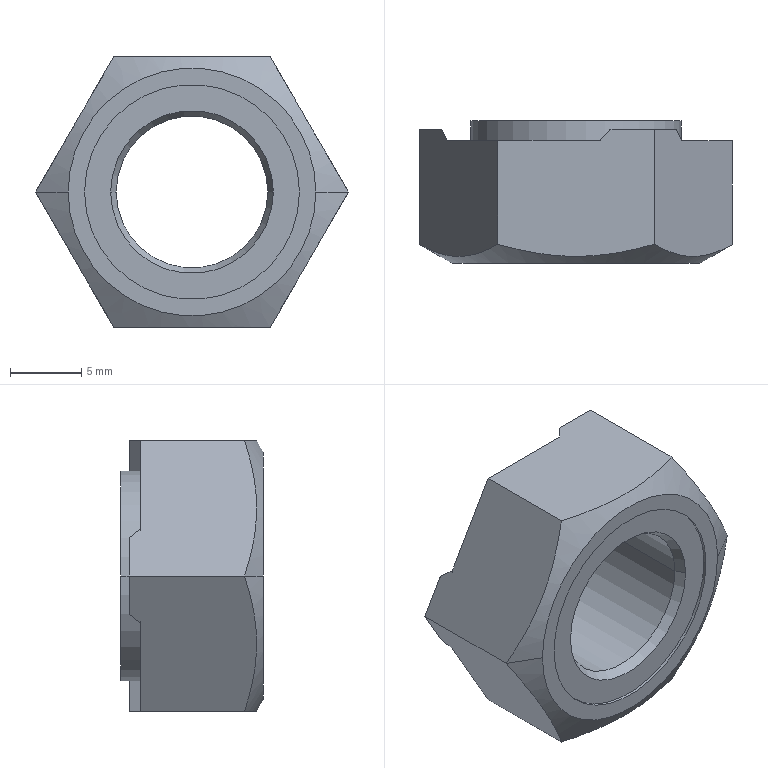Part | STEP file | _HEXAGON_WELD_NUTS_GB_-_-257103 | 1 solid | 28 faces | box 21.939 x 10 x 19 mm | volume 1991 mm3 | plane 16 | cone 6 | cylinder 6 | commonest cylinder face diameters 10.647 x2 14.75 x2 15.07 x2
STEP:
#1=CARTESIAN_POINT('',(-5.324,-14.533,-113.));
#2=VERTEX_POINT('',#1);
#3=CARTESIAN_POINT('',(5.324,-14.533,-113.));
#4=VERTEX_POINT('',#3);
#5=CARTESIAN_POINT('',(0.,-14.533,-113.));
#6=DIRECTION('',(0.,1.,0.));
#7=DIRECTION('',(-1.,0.,0.));
#8=AXIS2_PLACEMENT_3D('',#5,#6,#7);
#9=CIRCLE('',#8,5.324);
#10=EDGE_CURVE('',#2,#4,#9,.T.);
#11=ORIENTED_EDGE('',*,*,#10,.T.);
#12=CARTESIAN_POINT('',(5.708,-15.2,-113.));
#13=VERTEX_POINT('',#12);
#14=CARTESIAN_POINT('',(5.708,-15.2,-113.));
#15=DIRECTION('',(-0.5,0.866,0.));
#16=VECTOR('',#15,1000.);
#17=LINE('',#14,#16);
#18=EDGE_CURVE('',#13,#4,#17,.T.);
#19=ORIENTED_EDGE('',*,*,#18,.F.);
#20=CARTESIAN_POINT('',(-5.708,-15.2,-113.));
#21=VERTEX_POINT('',#20);
#22=CARTESIAN_POINT('',(0.,-15.2,-113.));
#23=DIRECTION('',(0.,1.,0.));
#24=DIRECTION('',(-1.,0.,0.));
#25=AXIS2_PLACEMENT_3D('',#22,#23,#24);
#26=CIRCLE('',#25,5.708);
#27=EDGE_CURVE('',#21,#13,#26,.T.);
#28=ORIENTED_EDGE('',*,*,#27,.F.);
#29=CARTESIAN_POINT('',(-5.708,-15.2,-113.));
#30=DIRECTION('',(0.5,0.866,0.));
#31=VECTOR('',#30,1000.);
#32=LINE('',#29,#31);
#33=EDGE_CURVE('',#21,#2,#32,.T.);
#34=ORIENTED_EDGE('',*,*,#33,.T.);
#35=EDGE_LOOP('',(#11,#19,#28,#34));
#36=FACE_OUTER_BOUND('',#35,.T.);
#37=CARTESIAN_POINT('',(0.,-14.867,-113.));
#38=DIRECTION('',(0.,-1.,0.));
#39=DIRECTION('',(1.,0.,0.));
#40=AXIS2_PLACEMENT_3D('',#37,#38,#39);
#41=CONICAL_SURFACE('',#40,5.516,0.5236);
#42=ADVANCED_FACE('',(#36),#41,.F.);
#43=CARTESIAN_POINT('',(-7.375,-6.8,-113.));
#44=VERTEX_POINT('',#43);
#45=CARTESIAN_POINT('',(7.375,-6.8,-113.));
#46=VERTEX_POINT('',#45);
#47=CARTESIAN_POINT('',(0.,-6.8,-113.));
#48=DIRECTION('',(0.,-1.,0.));
#49=DIRECTION('',(-1.,0.,0.));
#50=AXIS2_PLACEMENT_3D('',#47,#48,#49);
#51=CIRCLE('',#50,7.375);
#52=EDGE_CURVE('',#44,#46,#51,.T.);
#53=ORIENTED_EDGE('',*,*,#52,.F.);
#54=CARTESIAN_POINT('',(-7.375,-5.4,-113.));
#55=VERTEX_POINT('',#54);
#56=CARTESIAN_POINT('',(-7.375,-5.4,-113.));
#57=DIRECTION('',(0.,-1.,0.));
#58=VECTOR('',#57,1000.);
#59=LINE('',#56,#58);
#60=EDGE_CURVE('',#55,#44,#59,.T.);
#61=ORIENTED_EDGE('',*,*,#60,.F.);
#62=CARTESIAN_POINT('',(7.375,-5.4,-113.));
#63=VERTEX_POINT('',#62);
#64=CARTESIAN_POINT('',(0.,-5.4,-113.));
#65=DIRECTION('',(0.,1.,0.));
#66=DIRECTION('',(1.,0.,0.));
#67=AXIS2_PLACEMENT_3D('',#64,#65,#66);
#68=CIRCLE('',#67,7.375);
#69=EDGE_CURVE('',#63,#55,#68,.T.);
#70=ORIENTED_EDGE('',*,*,#69,.F.);
#71=CARTESIAN_POINT('',(7.375,-5.4,-113.));
#72=DIRECTION('',(0.,-1.,0.));
#73=VECTOR('',#72,1000.);
#74=LINE('',#71,#73);
#75=EDGE_CURVE('',#63,#46,#74,.T.);
#76=ORIENTED_EDGE('',*,*,#75,.T.);
#77=EDGE_LOOP('',(#53,#61,#70,#76));
#78=FACE_OUTER_BOUND('',#77,.T.);
#79=CARTESIAN_POINT('',(0.,-6.8,-113.));
#80=DIRECTION('',(0.,1.,0.));
#81=DIRECTION('',(-1.,0.,0.));
#82=AXIS2_PLACEMENT_3D('',#79,#80,#81);
#83=CYLINDRICAL_SURFACE('',#82,7.375);
#84=ADVANCED_FACE('',(#78),#83,.T.);
#85=CARTESIAN_POINT('',(-9.42,-6.,-110.315));
#86=VERTEX_POINT('',#85);
#87=CARTESIAN_POINT('',(-10.97,-6.,-113.));
#88=VERTEX_POINT('',#87);
#89=CARTESIAN_POINT('',(-9.42,-6.,-110.315));
#90=DIRECTION('',(-0.5,0.,-0.866));
#91=VECTOR('',#90,1000.);
#92=LINE('',#89,#91);
#93=EDGE_CURVE('',#86,#88,#92,.T.);
#94=ORIENTED_EDGE('',*,*,#93,.F.);
#95=CARTESIAN_POINT('',(-9.42,-6.,-115.685));
#96=VERTEX_POINT('',#95);
#97=CARTESIAN_POINT('',(-9.42,-6.,-110.315));
#98=DIRECTION('',(0.,0.,-1.));
#99=VECTOR('',#98,1000.);
#100=LINE('',#97,#99);
#101=EDGE_CURVE('',#86,#96,#100,.T.);
#102=ORIENTED_EDGE('',*,*,#101,.T.);
#103=CARTESIAN_POINT('',(-9.42,-6.,-115.685));
#104=DIRECTION('',(-0.5,0.,0.866));
#105=VECTOR('',#104,1000.);
#106=LINE('',#103,#105);
#107=EDGE_CURVE('',#96,#88,#106,.T.);
#108=ORIENTED_EDGE('',*,*,#107,.T.);
#109=EDGE_LOOP('',(#94,#102,#108));
#110=FACE_OUTER_BOUND('',#109,.T.);
#111=CARTESIAN_POINT('',(-10.97,-6.,-113.));
#112=DIRECTION('',(0.,1.,0.));
#113=DIRECTION('',(1.,0.,0.));
#114=AXIS2_PLACEMENT_3D('',#111,#112,#113);
#115=PLANE('',#114);
#116=ADVANCED_FACE('',(#110),#115,.T.);
#117=CARTESIAN_POINT('',(-9.047,-6.8,-116.331));
#118=VERTEX_POINT('',#117);
#119=CARTESIAN_POINT('',(-9.047,-6.8,-116.331));
#120=DIRECTION('',(-0.341,0.7313,0.5907));
#121=VECTOR('',#120,1000.);
#122=LINE('',#119,#121);
#123=EDGE_CURVE('',#118,#96,#122,.T.);
#124=ORIENTED_EDGE('',*,*,#123,.T.);
#125=ORIENTED_EDGE('',*,*,#101,.F.);
#126=CARTESIAN_POINT('',(-9.047,-6.8,-109.669));
#127=VERTEX_POINT('',#126);
#128=CARTESIAN_POINT('',(-9.047,-6.8,-109.669));
#129=DIRECTION('',(-0.341,0.7313,-0.5907));
#130=VECTOR('',#129,1000.);
#131=LINE('',#128,#130);
#132=EDGE_CURVE('',#127,#86,#131,.T.);
#133=ORIENTED_EDGE('',*,*,#132,.F.);
#134=CARTESIAN_POINT('',(-9.047,-6.8,-116.331));
#135=DIRECTION('',(0.,0.,1.));
#136=VECTOR('',#135,1000.);
#137=LINE('',#134,#136);
#138=EDGE_CURVE('',#118,#127,#137,.T.);
#139=ORIENTED_EDGE('',*,*,#138,.F.);
#140=EDGE_LOOP('',(#124,#125,#133,#139));
#141=FACE_OUTER_BOUND('',#140,.T.);
#142=CARTESIAN_POINT('',(-9.42,-6.,-110.315));
#143=DIRECTION('',(0.9063,0.4226,0.));
#144=DIRECTION('',(0.,0.,-1.));
#145=AXIS2_PLACEMENT_3D('',#142,#143,#144);
#146=PLANE('',#145);
#147=ADVANCED_FACE('',(#141),#146,.T.);
#148=CARTESIAN_POINT('',(7.035,-6.,-106.185));
#149=VERTEX_POINT('',#148);
#150=CARTESIAN_POINT('',(5.485,-6.,-103.5));
#151=VERTEX_POINT('',#150);
#152=CARTESIAN_POINT('',(7.035,-6.,-106.185));
#153=DIRECTION('',(-0.5,0.,0.866));
#154=VECTOR('',#153,1000.);
#155=LINE('',#152,#154);
#156=EDGE_CURVE('',#149,#151,#155,.T.);
#157=ORIENTED_EDGE('',*,*,#156,.F.);
#158=CARTESIAN_POINT('',(2.385,-6.,-103.5));
#159=VERTEX_POINT('',#158);
#160=CARTESIAN_POINT('',(7.035,-6.,-106.185));
#161=DIRECTION('',(-0.866,0.,0.5));
#162=VECTOR('',#161,1000.);
#163=LINE('',#160,#162);
#164=EDGE_CURVE('',#149,#159,#163,.T.);
#165=ORIENTED_EDGE('',*,*,#164,.T.);
#166=CARTESIAN_POINT('',(2.385,-6.,-103.5));
#167=DIRECTION('',(1.,0.,0.));
#168=VECTOR('',#167,1000.);
#169=LINE('',#166,#168);
#170=EDGE_CURVE('',#159,#151,#169,.T.);
#171=ORIENTED_EDGE('',*,*,#170,.T.);
#172=EDGE_LOOP('',(#157,#165,#171));
#173=FACE_OUTER_BOUND('',#172,.T.);
#174=CARTESIAN_POINT('',(5.485,-6.,-103.5));
#175=DIRECTION('',(0.,1.,0.));
#176=DIRECTION('',(1.,0.,0.));
#177=AXIS2_PLACEMENT_3D('',#174,#175,#176);
#178=PLANE('',#177);
#179=ADVANCED_FACE('',(#173),#178,.T.);
#180=CARTESIAN_POINT('',(1.639,-6.8,-103.5));
#181=VERTEX_POINT('',#180);
#182=CARTESIAN_POINT('',(1.639,-6.8,-103.5));
#183=DIRECTION('',(0.682,0.7313,0.));
#184=VECTOR('',#183,1000.);
#185=LINE('',#182,#184);
#186=EDGE_CURVE('',#181,#159,#185,.T.);
#187=ORIENTED_EDGE('',*,*,#186,.T.);
#188=ORIENTED_EDGE('',*,*,#164,.F.);
#189=CARTESIAN_POINT('',(7.408,-6.8,-106.831));
#190=VERTEX_POINT('',#189);
#191=CARTESIAN_POINT('',(7.408,-6.8,-106.831));
#192=DIRECTION('',(-0.341,0.7313,0.5907));
#193=VECTOR('',#192,1000.);
#194=LINE('',#191,#193);
#195=EDGE_CURVE('',#190,#149,#194,.T.);
#196=ORIENTED_EDGE('',*,*,#195,.F.);
#197=CARTESIAN_POINT('',(1.639,-6.8,-103.5));
#198=DIRECTION('',(0.866,0.,-0.5));
#199=VECTOR('',#198,1000.);
#200=LINE('',#197,#199);
#201=EDGE_CURVE('',#181,#190,#200,.T.);
#202=ORIENTED_EDGE('',*,*,#201,.F.);
#203=EDGE_LOOP('',(#187,#188,#196,#202));
#204=FACE_OUTER_BOUND('',#203,.T.);
#205=CARTESIAN_POINT('',(7.035,-6.,-106.185));
#206=DIRECTION('',(-0.4532,0.4226,-0.7849));
#207=DIRECTION('',(-0.866,0.,0.5));
#208=AXIS2_PLACEMENT_3D('',#205,#206,#207);
#209=PLANE('',#208);
#210=ADVANCED_FACE('',(#204),#209,.T.);
#211=CARTESIAN_POINT('',(2.385,-6.,-122.5));
#212=VERTEX_POINT('',#211);
#213=CARTESIAN_POINT('',(5.485,-6.,-122.5));
#214=VERTEX_POINT('',#213);
#215=CARTESIAN_POINT('',(2.385,-6.,-122.5));
#216=DIRECTION('',(1.,0.,0.));
#217=VECTOR('',#216,1000.);
#218=LINE('',#215,#217);
#219=EDGE_CURVE('',#212,#214,#218,.T.);
#220=ORIENTED_EDGE('',*,*,#219,.F.);
#221=CARTESIAN_POINT('',(7.035,-6.,-119.815));
#222=VERTEX_POINT('',#221);
#223=CARTESIAN_POINT('',(2.385,-6.,-122.5));
#224=DIRECTION('',(0.866,0.,0.5));
#225=VECTOR('',#224,1000.);
#226=LINE('',#223,#225);
#227=EDGE_CURVE('',#212,#222,#226,.T.);
#228=ORIENTED_EDGE('',*,*,#227,.T.);
#229=CARTESIAN_POINT('',(7.035,-6.,-119.815));
#230=DIRECTION('',(-0.5,0.,-0.866));
#231=VECTOR('',#230,1000.);
#232=LINE('',#229,#231);
#233=EDGE_CURVE('',#222,#214,#232,.T.);
#234=ORIENTED_EDGE('',*,*,#233,.T.);
#235=EDGE_LOOP('',(#220,#228,#234));
#236=FACE_OUTER_BOUND('',#235,.T.);
#237=CARTESIAN_POINT('',(5.485,-6.,-122.5));
#238=DIRECTION('',(0.,1.,0.));
#239=DIRECTION('',(1.,0.,0.));
#240=AXIS2_PLACEMENT_3D('',#237,#238,#239);
#241=PLANE('',#240);
#242=ADVANCED_FACE('',(#236),#241,.T.);
#243=CARTESIAN_POINT('',(7.408,-6.8,-119.169));
#244=VERTEX_POINT('',#243);
#245=CARTESIAN_POINT('',(7.408,-6.8,-119.169));
#246=DIRECTION('',(-0.341,0.7313,-0.5907));
#247=VECTOR('',#246,1000.);
#248=LINE('',#245,#247);
#249=EDGE_CURVE('',#244,#222,#248,.T.);
#250=ORIENTED_EDGE('',*,*,#249,.T.);
#251=ORIENTED_EDGE('',*,*,#227,.F.);
#252=CARTESIAN_POINT('',(1.639,-6.8,-122.5));
#253=VERTEX_POINT('',#252);
#254=CARTESIAN_POINT('',(1.639,-6.8,-122.5));
#255=DIRECTION('',(0.682,0.7313,0.));
#256=VECTOR('',#255,1000.);
#257=LINE('',#254,#256);
#258=EDGE_CURVE('',#253,#212,#257,.T.);
#259=ORIENTED_EDGE('',*,*,#258,.F.);
#260=CARTESIAN_POINT('',(7.408,-6.8,-119.169));
#261=DIRECTION('',(-0.866,0.,-0.5));
#262=VECTOR('',#261,1000.);
#263=LINE('',#260,#262);
#264=EDGE_CURVE('',#244,#253,#263,.T.);
#265=ORIENTED_EDGE('',*,*,#264,.F.);
#266=EDGE_LOOP('',(#250,#251,#259,#265));
#267=FACE_OUTER_BOUND('',#266,.T.);
#268=CARTESIAN_POINT('',(2.385,-6.,-122.5));
#269=DIRECTION('',(-0.4532,0.4226,0.7849));
#270=DIRECTION('',(0.682,0.7313,0.));
#271=AXIS2_PLACEMENT_3D('',#268,#269,#270);
#272=PLANE('',#271);
#273=ADVANCED_FACE('',(#267),#272,.T.);
#274=ORIENTED_EDGE('',*,*,#52,.T.);
#275=CARTESIAN_POINT('',(0.,-6.8,-113.));
#276=DIRECTION('',(0.,-1.,0.));
#277=DIRECTION('',(1.,0.,0.));
#278=AXIS2_PLACEMENT_3D('',#275,#276,#277);
#279=CIRCLE('',#278,7.375);
#280=EDGE_CURVE('',#46,#44,#279,.T.);
#281=ORIENTED_EDGE('',*,*,#280,.T.);
#282=EDGE_LOOP('',(#274,#281));
#283=FACE_BOUND('',#282,.T.);
#284=ORIENTED_EDGE('',*,*,#138,.T.);
#285=CARTESIAN_POINT('',(-5.485,-6.8,-103.5));
#286=VERTEX_POINT('',#285);
#287=CARTESIAN_POINT('',(-9.047,-6.8,-109.669));
#288=DIRECTION('',(0.5,0.,0.866));
#289=VECTOR('',#288,1000.);
#290=LINE('',#287,#289);
#291=EDGE_CURVE('',#127,#286,#290,.T.);
#292=ORIENTED_EDGE('',*,*,#291,.T.);
#293=CARTESIAN_POINT('',(-5.485,-6.8,-103.5));
#294=DIRECTION('',(1.,0.,0.));
#295=VECTOR('',#294,1000.);
#296=LINE('',#293,#295);
#297=EDGE_CURVE('',#286,#181,#296,.T.);
#298=ORIENTED_EDGE('',*,*,#297,.T.);
#299=ORIENTED_EDGE('',*,*,#201,.T.);
#300=CARTESIAN_POINT('',(10.97,-6.8,-113.));
#301=VERTEX_POINT('',#300);
#302=CARTESIAN_POINT('',(7.408,-6.8,-106.831));
#303=DIRECTION('',(0.5,0.,-0.866));
#304=VECTOR('',#303,1000.);
#305=LINE('',#302,#304);
#306=EDGE_CURVE('',#190,#301,#305,.T.);
#307=ORIENTED_EDGE('',*,*,#306,.T.);
#308=CARTESIAN_POINT('',(10.97,-6.8,-113.));
#309=DIRECTION('',(-0.5,0.,-0.866));
#310=VECTOR('',#309,1000.);
#311=LINE('',#308,#310);
#312=EDGE_CURVE('',#301,#244,#311,.T.);
#313=ORIENTED_EDGE('',*,*,#312,.T.);
#314=ORIENTED_EDGE('',*,*,#264,.T.);
#315=CARTESIAN_POINT('',(-5.485,-6.8,-122.5));
#316=VERTEX_POINT('',#315);
#317=CARTESIAN_POINT('',(1.639,-6.8,-122.5));
#318=DIRECTION('',(-1.,0.,0.));
#319=VECTOR('',#318,1000.);
#320=LINE('',#317,#319);
#321=EDGE_CURVE('',#253,#316,#320,.T.);
#322=ORIENTED_EDGE('',*,*,#321,.T.);
#323=CARTESIAN_POINT('',(-5.485,-6.8,-122.5));
#324=DIRECTION('',(-0.5,0.,0.866));
#325=VECTOR('',#324,1000.);
#326=LINE('',#323,#325);
#327=EDGE_CURVE('',#316,#118,#326,.T.);
#328=ORIENTED_EDGE('',*,*,#327,.T.);
#329=EDGE_LOOP('',(#284,#292,#298,#299,#307,#313,#314,#322,#328));
#330=FACE_OUTER_BOUND('',#329,.T.);
#331=CARTESIAN_POINT('',(0.,-6.8,-113.));
#332=DIRECTION('',(0.,1.,0.));
#333=DIRECTION('',(1.,0.,0.));
#334=AXIS2_PLACEMENT_3D('',#331,#332,#333);
#335=PLANE('',#334);
#336=ADVANCED_FACE('',(#283,#330),#335,.T.);
#337=ORIENTED_EDGE('',*,*,#75,.F.);
#338=CARTESIAN_POINT('',(0.,-5.4,-113.));
#339=DIRECTION('',(0.,1.,0.));
#340=DIRECTION('',(-1.,0.,0.));
#341=AXIS2_PLACEMENT_3D('',#338,#339,#340);
#342=CIRCLE('',#341,7.375);
#343=EDGE_CURVE('',#55,#63,#342,.T.);
#344=ORIENTED_EDGE('',*,*,#343,.F.);
#345=ORIENTED_EDGE('',*,*,#60,.T.);
#346=ORIENTED_EDGE('',*,*,#280,.F.);
#347=EDGE_LOOP('',(#337,#344,#345,#346));
#348=FACE_OUTER_BOUND('',#347,.T.);
#349=CARTESIAN_POINT('',(0.,-6.8,-113.));
#350=DIRECTION('',(0.,1.,0.));
#351=DIRECTION('',(-1.,0.,0.));
#352=AXIS2_PLACEMENT_3D('',#349,#350,#351);
#353=CYLINDRICAL_SURFACE('',#352,7.375);
#354=ADVANCED_FACE('',(#348),#353,.T.);
#355=CARTESIAN_POINT('',(5.99,-5.4,-113.));
#356=VERTEX_POINT('',#355);
#357=CARTESIAN_POINT('',(-5.99,-5.4,-113.));
#358=VERTEX_POINT('',#357);
#359=CARTESIAN_POINT('',(0.,-5.4,-113.));
#360=DIRECTION('',(0.,-1.,0.));
#361=DIRECTION('',(1.,0.,0.));
#362=AXIS2_PLACEMENT_3D('',#359,#360,#361);
#363=CIRCLE('',#362,5.99);
#364=EDGE_CURVE('',#356,#358,#363,.T.);
#365=ORIENTED_EDGE('',*,*,#364,.T.);
#366=CARTESIAN_POINT('',(0.,-5.4,-113.));
#367=DIRECTION('',(0.,-1.,0.));
#368=DIRECTION('',(-1.,0.,0.));
#369=AXIS2_PLACEMENT_3D('',#366,#367,#368);
#370=CIRCLE('',#369,5.99);
#371=EDGE_CURVE('',#358,#356,#370,.T.);
#372=ORIENTED_EDGE('',*,*,#371,.T.);
#373=EDGE_LOOP('',(#365,#372));
#374=FACE_BOUND('',#373,.T.);
#375=ORIENTED_EDGE('',*,*,#69,.T.);
#376=ORIENTED_EDGE('',*,*,#343,.T.);
#377=EDGE_LOOP('',(#375,#376));
#378=FACE_OUTER_BOUND('',#377,.T.);
#379=CARTESIAN_POINT('',(5.485,-5.4,-122.5));
#380=DIRECTION('',(0.,-1.,0.));
#381=DIRECTION('',(0.,0.,-1.));
#382=AXIS2_PLACEMENT_3D('',#379,#380,#381);
#383=PLANE('',#382);
#384=ADVANCED_FACE('',(#374,#378),#383,.F.);
#385=CARTESIAN_POINT('',(5.324,-5.785,-113.));
#386=VERTEX_POINT('',#385);
#387=CARTESIAN_POINT('',(5.99,-5.4,-113.));
#388=DIRECTION('',(-0.866,-0.5,0.));
#389=VECTOR('',#388,1000.);
#390=LINE('',#387,#389);
#391=EDGE_CURVE('',#356,#386,#390,.T.);
#392=ORIENTED_EDGE('',*,*,#391,.F.);
#393=ORIENTED_EDGE('',*,*,#371,.F.);
#394=CARTESIAN_POINT('',(-5.324,-5.785,-113.));
#395=VERTEX_POINT('',#394);
#396=CARTESIAN_POINT('',(-5.99,-5.4,-113.));
#397=DIRECTION('',(0.866,-0.5,0.));
#398=VECTOR('',#397,1000.);
#399=LINE('',#396,#398);
#400=EDGE_CURVE('',#358,#395,#399,.T.);
#401=ORIENTED_EDGE('',*,*,#400,.T.);
#402=CARTESIAN_POINT('',(0.,-5.785,-113.));
#403=DIRECTION('',(0.,-1.,0.));
#404=DIRECTION('',(-1.,0.,0.));
#405=AXIS2_PLACEMENT_3D('',#402,#403,#404);
#406=CIRCLE('',#405,5.324);
#407=EDGE_CURVE('',#395,#386,#406,.T.);
#408=ORIENTED_EDGE('',*,*,#407,.T.);
#409=EDGE_LOOP('',(#392,#393,#401,#408));
#410=FACE_OUTER_BOUND('',#409,.T.);
#411=CARTESIAN_POINT('',(0.,-5.592,-113.));
#412=DIRECTION('',(0.,1.,0.));
#413=DIRECTION('',(-1.,0.,0.));
#414=AXIS2_PLACEMENT_3D('',#411,#412,#413);
#415=CONICAL_SURFACE('',#414,5.657,1.047);
#416=ADVANCED_FACE('',(#410),#415,.F.);
#417=CARTESIAN_POINT('',(0.,-5.785,-113.));
#418=DIRECTION('',(0.,-1.,0.));
#419=DIRECTION('',(1.,0.,0.));
#420=AXIS2_PLACEMENT_3D('',#417,#418,#419);
#421=CIRCLE('',#420,5.324);
#422=EDGE_CURVE('',#386,#395,#421,.T.);
#423=ORIENTED_EDGE('',*,*,#422,.T.);
#424=ORIENTED_EDGE('',*,*,#400,.F.);
#425=ORIENTED_EDGE('',*,*,#364,.F.);
#426=ORIENTED_EDGE('',*,*,#391,.T.);
#427=EDGE_LOOP('',(#423,#424,#425,#426));
#428=FACE_OUTER_BOUND('',#427,.T.);
#429=CARTESIAN_POINT('',(0.,-5.592,-113.));
#430=DIRECTION('',(0.,1.,0.));
#431=DIRECTION('',(-1.,0.,0.));
#432=AXIS2_PLACEMENT_3D('',#429,#430,#431);
#433=CONICAL_SURFACE('',#432,5.657,1.047);
#434=ADVANCED_FACE('',(#428),#433,.F.);
#435=ORIENTED_EDGE('',*,*,#10,.F.);
#436=CARTESIAN_POINT('',(-5.324,-5.785,-113.));
#437=DIRECTION('',(0.,-1.,0.));
#438=VECTOR('',#437,1000.);
#439=LINE('',#436,#438);
#440=EDGE_CURVE('',#395,#2,#439,.T.);
#441=ORIENTED_EDGE('',*,*,#440,.F.);
#442=ORIENTED_EDGE('',*,*,#422,.F.);
#443=CARTESIAN_POINT('',(5.324,-5.785,-113.));
#444=DIRECTION('',(0.,-1.,0.));
#445=VECTOR('',#444,1000.);
#446=LINE('',#443,#445);
#447=EDGE_CURVE('',#386,#4,#446,.T.);
#448=ORIENTED_EDGE('',*,*,#447,.T.);
#449=EDGE_LOOP('',(#435,#441,#442,#448));
#450=FACE_OUTER_BOUND('',#449,.T.);
#451=CARTESIAN_POINT('',(0.,-15.4,-113.));
#452=DIRECTION('',(0.,1.,0.));
#453=DIRECTION('',(-1.,0.,0.));
#454=AXIS2_PLACEMENT_3D('',#451,#452,#453);
#455=CYLINDRICAL_SURFACE('',#454,5.324);
#456=ADVANCED_FACE('',(#450),#455,.F.);
#457=ORIENTED_EDGE('',*,*,#447,.F.);
#458=ORIENTED_EDGE('',*,*,#407,.F.);
#459=ORIENTED_EDGE('',*,*,#440,.T.);
#460=CARTESIAN_POINT('',(0.,-14.533,-113.));
#461=DIRECTION('',(0.,1.,0.));
#462=DIRECTION('',(1.,0.,0.));
#463=AXIS2_PLACEMENT_3D('',#460,#461,#462);
#464=CIRCLE('',#463,5.324);
#465=EDGE_CURVE('',#4,#2,#464,.T.);
#466=ORIENTED_EDGE('',*,*,#465,.F.);
#467=EDGE_LOOP('',(#457,#458,#459,#466));
#468=FACE_OUTER_BOUND('',#467,.T.);
#469=CARTESIAN_POINT('',(0.,-15.4,-113.));
#470=DIRECTION('',(0.,1.,0.));
#471=DIRECTION('',(-1.,0.,0.));
#472=AXIS2_PLACEMENT_3D('',#469,#470,#471);
#473=CYLINDRICAL_SURFACE('',#472,5.324);
#474=ADVANCED_FACE('',(#468),#473,.F.);
#475=ORIENTED_EDGE('',*,*,#33,.F.);
#476=CARTESIAN_POINT('',(0.,-15.2,-113.));
#477=DIRECTION('',(0.,1.,0.));
#478=DIRECTION('',(1.,0.,0.));
#479=AXIS2_PLACEMENT_3D('',#476,#477,#478);
#480=CIRCLE('',#479,5.708);
#481=EDGE_CURVE('',#13,#21,#480,.T.);
#482=ORIENTED_EDGE('',*,*,#481,.F.);
#483=ORIENTED_EDGE('',*,*,#18,.T.);
#484=ORIENTED_EDGE('',*,*,#465,.T.);
#485=EDGE_LOOP('',(#475,#482,#483,#484));
#486=FACE_OUTER_BOUND('',#485,.T.);
#487=CARTESIAN_POINT('',(0.,-14.867,-113.));
#488=DIRECTION('',(0.,-1.,0.));
#489=DIRECTION('',(1.,0.,0.));
#490=AXIS2_PLACEMENT_3D('',#487,#488,#489);
#491=CONICAL_SURFACE('',#490,5.516,0.5236);
#492=ADVANCED_FACE('',(#486),#491,.F.);
#493=ORIENTED_EDGE('',*,*,#27,.T.);
#494=ORIENTED_EDGE('',*,*,#481,.T.);
#495=EDGE_LOOP('',(#493,#494));
#496=FACE_BOUND('',#495,.T.);
#497=CARTESIAN_POINT('',(-7.535,-15.2,-113.));
#498=VERTEX_POINT('',#497);
#499=CARTESIAN_POINT('',(7.535,-15.2,-113.));
#500=VERTEX_POINT('',#499);
#501=CARTESIAN_POINT('',(0.,-15.2,-113.));
#502=DIRECTION('',(0.,-1.,0.));
#503=DIRECTION('',(-1.,0.,0.));
#504=AXIS2_PLACEMENT_3D('',#501,#502,#503);
#505=CIRCLE('',#504,7.535);
#506=EDGE_CURVE('',#498,#500,#505,.T.);
#507=ORIENTED_EDGE('',*,*,#506,.T.);
#508=CARTESIAN_POINT('',(0.,-15.2,-113.));
#509=DIRECTION('',(0.,-1.,0.));
#510=DIRECTION('',(1.,0.,0.));
#511=AXIS2_PLACEMENT_3D('',#508,#509,#510);
#512=CIRCLE('',#511,7.535);
#513=EDGE_CURVE('',#500,#498,#512,.T.);
#514=ORIENTED_EDGE('',*,*,#513,.T.);
#515=EDGE_LOOP('',(#507,#514));
#516=FACE_OUTER_BOUND('',#515,.T.);
#517=CARTESIAN_POINT('',(0.,-15.2,-113.));
#518=DIRECTION('',(0.,1.,0.));
#519=DIRECTION('',(1.,0.,0.));
#520=AXIS2_PLACEMENT_3D('',#517,#518,#519);
#521=PLANE('',#520);
#522=ADVANCED_FACE('',(#496,#516),#521,.F.);
#523=CARTESIAN_POINT('',(7.535,-15.4,-113.));
#524=VERTEX_POINT('',#523);
#525=CARTESIAN_POINT('',(7.535,-15.2,-113.));
#526=DIRECTION('',(0.,-1.,0.));
#527=VECTOR('',#526,1000.);
#528=LINE('',#525,#527);
#529=EDGE_CURVE('',#500,#524,#528,.T.);
#530=ORIENTED_EDGE('',*,*,#529,.F.);
#531=ORIENTED_EDGE('',*,*,#506,.F.);
#532=CARTESIAN_POINT('',(-7.535,-15.4,-113.));
#533=VERTEX_POINT('',#532);
#534=CARTESIAN_POINT('',(-7.535,-15.2,-113.));
#535=DIRECTION('',(0.,-1.,0.));
#536=VECTOR('',#535,1000.);
#537=LINE('',#534,#536);
#538=EDGE_CURVE('',#498,#533,#537,.T.);
#539=ORIENTED_EDGE('',*,*,#538,.T.);
#540=CARTESIAN_POINT('',(0.,-15.4,-113.));
#541=DIRECTION('',(0.,1.,0.));
#542=DIRECTION('',(1.,0.,0.));
#543=AXIS2_PLACEMENT_3D('',#540,#541,#542);
#544=CIRCLE('',#543,7.535);
#545=EDGE_CURVE('',#524,#533,#544,.T.);
#546=ORIENTED_EDGE('',*,*,#545,.F.);
#547=EDGE_LOOP('',(#530,#531,#539,#546));
#548=FACE_OUTER_BOUND('',#547,.T.);
#549=CARTESIAN_POINT('',(0.,-5.498,-113.));
#550=DIRECTION('',(0.,1.,0.));
#551=DIRECTION('',(-1.,0.,0.));
#552=AXIS2_PLACEMENT_3D('',#549,#550,#551);
#553=CYLINDRICAL_SURFACE('',#552,7.535);
#554=ADVANCED_FACE('',(#548),#553,.F.);
#555=CARTESIAN_POINT('',(0.,-15.4,-113.));
#556=DIRECTION('',(0.,1.,0.));
#557=DIRECTION('',(-1.,0.,0.));
#558=AXIS2_PLACEMENT_3D('',#555,#556,#557);
#559=CIRCLE('',#558,7.535);
#560=EDGE_CURVE('',#533,#524,#559,.T.);
#561=ORIENTED_EDGE('',*,*,#560,.F.);
#562=ORIENTED_EDGE('',*,*,#538,.F.);
#563=ORIENTED_EDGE('',*,*,#513,.F.);
#564=ORIENTED_EDGE('',*,*,#529,.T.);
#565=EDGE_LOOP('',(#561,#562,#563,#564));
#566=FACE_OUTER_BOUND('',#565,.T.);
#567=CARTESIAN_POINT('',(0.,-5.498,-113.));
#568=DIRECTION('',(0.,1.,0.));
#569=DIRECTION('',(-1.,0.,0.));
#570=AXIS2_PLACEMENT_3D('',#567,#568,#569);
#571=CYLINDRICAL_SURFACE('',#570,7.535);
#572=ADVANCED_FACE('',(#566),#571,.F.);
#573=ORIENTED_EDGE('',*,*,#545,.T.);
#574=ORIENTED_EDGE('',*,*,#560,.T.);
#575=EDGE_LOOP('',(#573,#574));
#576=FACE_BOUND('',#575,.T.);
#577=CARTESIAN_POINT('',(-8.685,-15.4,-113.));
#578=VERTEX_POINT('',#577);
#579=CARTESIAN_POINT('',(8.685,-15.4,-113.));
#580=VERTEX_POINT('',#579);
#581=CARTESIAN_POINT('',(0.,-15.4,-113.));
#582=DIRECTION('',(0.,-1.,0.));
#583=DIRECTION('',(-1.,0.,0.));
#584=AXIS2_PLACEMENT_3D('',#581,#582,#583);
#585=CIRCLE('',#584,8.685);
#586=EDGE_CURVE('',#578,#580,#585,.T.);
#587=ORIENTED_EDGE('',*,*,#586,.T.);
#588=CARTESIAN_POINT('',(0.,-15.4,-113.));
#589=DIRECTION('',(0.,-1.,0.));
#590=DIRECTION('',(1.,0.,0.));
#591=AXIS2_PLACEMENT_3D('',#588,#589,#590);
#592=CIRCLE('',#591,8.685);
#593=EDGE_CURVE('',#580,#578,#592,.T.);
#594=ORIENTED_EDGE('',*,*,#593,.T.);
#595=EDGE_LOOP('',(#587,#594));
#596=FACE_OUTER_BOUND('',#595,.T.);
#597=CARTESIAN_POINT('',(5.485,-15.4,-122.5));
#598=DIRECTION('',(0.,-1.,0.));
#599=DIRECTION('',(0.,0.,-1.));
#600=AXIS2_PLACEMENT_3D('',#597,#598,#599);
#601=PLANE('',#600);
#602=ADVANCED_FACE('',(#576,#596),#601,.T.);
#603=CARTESIAN_POINT('',(10.97,-14.081,-113.));
#604=VERTEX_POINT('',#603);
#605=CARTESIAN_POINT('',(10.97,-14.081,-113.));
#606=DIRECTION('',(-0.866,-0.5,0.));
#607=VECTOR('',#606,1000.);
#608=LINE('',#605,#607);
#609=EDGE_CURVE('',#604,#580,#608,.T.);
#610=ORIENTED_EDGE('',*,*,#609,.F.);
#611=CARTESIAN_POINT('',(5.485,-14.081,-103.5));
#612=VERTEX_POINT('',#611);
#613=CARTESIAN_POINT('',(10.97,-14.081,-113.));
#614=CARTESIAN_POINT('',(10.732,-14.218,-112.589));
#615=CARTESIAN_POINT('',(10.5,-14.339,-112.188));
#616=CARTESIAN_POINT('',(10.158,-14.495,-111.594));
#617=CARTESIAN_POINT('',(10.044,-14.543,-111.397));
#618=CARTESIAN_POINT('',(9.875,-14.609,-111.104));
#619=CARTESIAN_POINT('',(9.818,-14.63,-111.006));
#620=CARTESIAN_POINT('',(9.706,-14.67,-110.811));
#621=CARTESIAN_POINT('',(9.651,-14.689,-110.715));
#622=CARTESIAN_POINT('',(9.479,-14.744,-110.418));
#623=CARTESIAN_POINT('',(9.365,-14.776,-110.221));
#624=CARTESIAN_POINT('',(9.138,-14.831,-109.827));
#625=CARTESIAN_POINT('',(9.026,-14.854,-109.633));
#626=CARTESIAN_POINT('',(8.683,-14.91,-109.039));
#627=CARTESIAN_POINT('',(8.458,-14.929,-108.649));
#628=CARTESIAN_POINT('',(8.114,-14.929,-108.054));
#629=CARTESIAN_POINT('',(8.,-14.925,-107.857));
#630=CARTESIAN_POINT('',(7.829,-14.911,-107.56));
#631=CARTESIAN_POINT('',(7.772,-14.905,-107.461));
#632=CARTESIAN_POINT('',(7.657,-14.89,-107.263));
#633=CARTESIAN_POINT('',(7.599,-14.882,-107.162));
#634=CARTESIAN_POINT('',(7.429,-14.854,-106.867));
#635=CARTESIAN_POINT('',(7.315,-14.831,-106.671));
#636=CARTESIAN_POINT('',(7.145,-14.789,-106.375));
#637=CARTESIAN_POINT('',(7.059,-14.767,-106.227));
#638=CARTESIAN_POINT('',(6.974,-14.742,-106.079));
#639=CARTESIAN_POINT('',(6.916,-14.725,-105.979));
#640=CARTESIAN_POINT('',(6.887,-14.715,-105.929));
#641=CARTESIAN_POINT('',(6.41,-14.563,-105.102));
#642=CARTESIAN_POINT('',(5.958,-14.354,-104.32));
#643=CARTESIAN_POINT('',(5.485,-14.081,-103.5));
#644=B_SPLINE_CURVE_WITH_KNOTS('',3,(#613,#614,#615,#616,#617,#618,#619,#620,#621,#622,#623,#624,#625,#626,#627,#628,#629,#630,#631,#632,#633,#634,#635,#636,#637,#638,#639,#640,#641,#642,#643),.UNSPECIFIED.,.F.,.F.,(4,2,2,2,2,2,2,2,2,2,2,2,1,2,2,4),(0.,0.125,0.1875,0.2187,0.25,0.3125,0.375,0.5,0.5625,0.5937,0.625,0.6875,0.7187,0.7344,0.75,1.),.UNSPECIFIED.);
#645=EDGE_CURVE('',#604,#612,#644,.T.);
#646=ORIENTED_EDGE('',*,*,#645,.T.);
#647=CARTESIAN_POINT('',(-5.485,-14.081,-103.5));
#648=VERTEX_POINT('',#647);
#649=CARTESIAN_POINT('',(5.485,-14.081,-103.5));
#650=CARTESIAN_POINT('',(5.011,-14.218,-103.5));
#651=CARTESIAN_POINT('',(4.549,-14.338,-103.5));
#652=CARTESIAN_POINT('',(3.864,-14.494,-103.5));
#653=CARTESIAN_POINT('',(3.638,-14.542,-103.5));
#654=CARTESIAN_POINT('',(3.3,-14.608,-103.5));
#655=CARTESIAN_POINT('',(3.131,-14.64,-103.5));
#656=CARTESIAN_POINT('',(2.962,-14.669,-103.5));
#657=CARTESIAN_POINT('',(2.85,-14.688,-103.5));
#658=CARTESIAN_POINT('',(2.796,-14.697,-103.5));
#659=CARTESIAN_POINT('',(2.275,-14.78,-103.5));
#660=CARTESIAN_POINT('',(1.821,-14.836,-103.5));
#661=CARTESIAN_POINT('',(1.132,-14.892,-103.5));
#662=CARTESIAN_POINT('',(0.9033,-14.906,-103.5));
#663=CARTESIAN_POINT('',(0.4471,-14.925,-103.5));
#664=CARTESIAN_POINT('',(0.2179,-14.93,-103.5));
#665=CARTESIAN_POINT('',(-0.2369,-14.929,-103.5));
#666=CARTESIAN_POINT('',(-0.4634,-14.925,-103.5));
#667=CARTESIAN_POINT('',(-0.917,-14.906,-103.5));
#668=CARTESIAN_POINT('',(-1.146,-14.891,-103.5));
#669=CARTESIAN_POINT('',(-1.599,-14.854,-103.5));
#670=CARTESIAN_POINT('',(-1.825,-14.831,-103.5));
#671=CARTESIAN_POINT('',(-2.164,-14.789,-103.5));
#672=CARTESIAN_POINT('',(-2.278,-14.774,-103.5));
#673=CARTESIAN_POINT('',(-2.505,-14.742,-103.5));
#674=CARTESIAN_POINT('',(-2.621,-14.725,-103.5));
#675=CARTESIAN_POINT('',(-3.633,-14.563,-103.5));
#676=CARTESIAN_POINT('',(-4.537,-14.355,-103.5));
#677=CARTESIAN_POINT('',(-5.485,-14.081,-103.5));
#678=B_SPLINE_CURVE_WITH_KNOTS('',3,(#649,#650,#651,#652,#653,#654,#655,#656,#657,#658,#659,#660,#661,#662,#663,#664,#665,#666,#667,#668,#669,#670,#671,#672,#673,#674,#675,#676,#677),.UNSPECIFIED.,.F.,.F.,(4,2,2,1,2,2,2,2,2,2,2,2,2,2,4),(0.,0.125,0.1875,0.2188,0.2344,0.25,0.375,0.4375,0.5,0.5625,0.625,0.6875,0.7188,0.75,1.),.UNSPECIFIED.);
#679=EDGE_CURVE('',#612,#648,#678,.T.);
#680=ORIENTED_EDGE('',*,*,#679,.T.);
#681=CARTESIAN_POINT('',(-10.97,-14.081,-113.));
#682=VERTEX_POINT('',#681);
#683=CARTESIAN_POINT('',(-5.485,-14.081,-103.5));
#684=CARTESIAN_POINT('',(-5.722,-14.218,-103.911));
#685=CARTESIAN_POINT('',(-5.954,-14.339,-104.313));
#686=CARTESIAN_POINT('',(-6.296,-14.495,-104.906));
#687=CARTESIAN_POINT('',(-6.41,-14.543,-105.103));
#688=CARTESIAN_POINT('',(-6.58,-14.609,-105.396));
#689=CARTESIAN_POINT('',(-6.636,-14.63,-105.494));
#690=CARTESIAN_POINT('',(-6.749,-14.67,-105.689));
#691=CARTESIAN_POINT('',(-6.804,-14.689,-105.785));
#692=CARTESIAN_POINT('',(-6.976,-14.744,-106.082));
#693=CARTESIAN_POINT('',(-7.09,-14.776,-106.279));
#694=CARTESIAN_POINT('',(-7.316,-14.831,-106.672));
#695=CARTESIAN_POINT('',(-7.429,-14.854,-106.867));
#696=CARTESIAN_POINT('',(-7.772,-14.91,-107.461));
#697=CARTESIAN_POINT('',(-7.997,-14.929,-107.851));
#698=CARTESIAN_POINT('',(-8.34,-14.929,-108.446));
#699=CARTESIAN_POINT('',(-8.454,-14.925,-108.643));
#700=CARTESIAN_POINT('',(-8.626,-14.911,-108.94));
#701=CARTESIAN_POINT('',(-8.683,-14.905,-109.039));
#702=CARTESIAN_POINT('',(-8.797,-14.89,-109.237));
#703=CARTESIAN_POINT('',(-8.855,-14.882,-109.338));
#704=CARTESIAN_POINT('',(-9.026,-14.854,-109.633));
#705=CARTESIAN_POINT('',(-9.139,-14.831,-109.829));
#706=CARTESIAN_POINT('',(-9.31,-14.789,-110.125));
#707=CARTESIAN_POINT('',(-9.395,-14.767,-110.273));
#708=CARTESIAN_POINT('',(-9.481,-14.742,-110.421));
#709=CARTESIAN_POINT('',(-9.538,-14.725,-110.521));
#710=CARTESIAN_POINT('',(-9.567,-14.715,-110.571));
#711=CARTESIAN_POINT('',(-10.045,-14.563,-111.398));
#712=CARTESIAN_POINT('',(-10.496,-14.354,-112.18));
#713=CARTESIAN_POINT('',(-10.97,-14.081,-113.));
#714=B_SPLINE_CURVE_WITH_KNOTS('',3,(#683,#684,#685,#686,#687,#688,#689,#690,#691,#692,#693,#694,#695,#696,#697,#698,#699,#700,#701,#702,#703,#704,#705,#706,#707,#708,#709,#710,#711,#712,#713),.UNSPECIFIED.,.F.,.F.,(4,2,2,2,2,2,2,2,2,2,2,2,1,2,2,4),(0.,0.125,0.1875,0.2187,0.25,0.3125,0.375,0.5,0.5625,0.5937,0.625,0.6875,0.7187,0.7344,0.75,1.),.UNSPECIFIED.);
#715=EDGE_CURVE('',#648,#682,#714,.T.);
#716=ORIENTED_EDGE('',*,*,#715,.T.);
#717=CARTESIAN_POINT('',(-10.97,-14.081,-113.));
#718=DIRECTION('',(0.866,-0.5,0.));
#719=VECTOR('',#718,1000.);
#720=LINE('',#717,#719);
#721=EDGE_CURVE('',#682,#578,#720,.T.);
#722=ORIENTED_EDGE('',*,*,#721,.T.);
#723=ORIENTED_EDGE('',*,*,#593,.F.);
#724=EDGE_LOOP('',(#610,#646,#680,#716,#722,#723));
#725=FACE_OUTER_BOUND('',#724,.T.);
#726=CARTESIAN_POINT('',(0.,-14.74,-113.));
#727=DIRECTION('',(0.,1.,0.));
#728=DIRECTION('',(-1.,0.,0.));
#729=AXIS2_PLACEMENT_3D('',#726,#727,#728);
#730=CONICAL_SURFACE('',#729,9.827,1.047);
#731=ADVANCED_FACE('',(#725),#730,.T.);
#732=ORIENTED_EDGE('',*,*,#586,.F.);
#733=ORIENTED_EDGE('',*,*,#721,.F.);
#734=CARTESIAN_POINT('',(-5.485,-14.081,-122.5));
#735=VERTEX_POINT('',#734);
#736=CARTESIAN_POINT('',(-10.97,-14.081,-113.));
#737=CARTESIAN_POINT('',(-10.732,-14.218,-113.411));
#738=CARTESIAN_POINT('',(-10.5,-14.339,-113.812));
#739=CARTESIAN_POINT('',(-10.158,-14.495,-114.406));
#740=CARTESIAN_POINT('',(-10.044,-14.543,-114.603));
#741=CARTESIAN_POINT('',(-9.875,-14.609,-114.896));
#742=CARTESIAN_POINT('',(-9.818,-14.63,-114.994));
#743=CARTESIAN_POINT('',(-9.706,-14.67,-115.189));
#744=CARTESIAN_POINT('',(-9.651,-14.689,-115.285));
#745=CARTESIAN_POINT('',(-9.479,-14.744,-115.582));
#746=CARTESIAN_POINT('',(-9.365,-14.776,-115.779));
#747=CARTESIAN_POINT('',(-9.138,-14.831,-116.173));
#748=CARTESIAN_POINT('',(-9.026,-14.854,-116.367));
#749=CARTESIAN_POINT('',(-8.683,-14.91,-116.961));
#750=CARTESIAN_POINT('',(-8.458,-14.929,-117.351));
#751=CARTESIAN_POINT('',(-8.114,-14.929,-117.946));
#752=CARTESIAN_POINT('',(-8.,-14.925,-118.143));
#753=CARTESIAN_POINT('',(-7.829,-14.911,-118.44));
#754=CARTESIAN_POINT('',(-7.772,-14.905,-118.539));
#755=CARTESIAN_POINT('',(-7.657,-14.89,-118.737));
#756=CARTESIAN_POINT('',(-7.599,-14.882,-118.838));
#757=CARTESIAN_POINT('',(-7.429,-14.854,-119.133));
#758=CARTESIAN_POINT('',(-7.315,-14.831,-119.329));
#759=CARTESIAN_POINT('',(-7.145,-14.789,-119.625));
#760=CARTESIAN_POINT('',(-7.059,-14.767,-119.773));
#761=CARTESIAN_POINT('',(-6.974,-14.742,-119.921));
#762=CARTESIAN_POINT('',(-6.916,-14.725,-120.021));
#763=CARTESIAN_POINT('',(-6.887,-14.715,-120.071));
#764=CARTESIAN_POINT('',(-6.41,-14.563,-120.898));
#765=CARTESIAN_POINT('',(-5.958,-14.354,-121.68));
#766=CARTESIAN_POINT('',(-5.485,-14.081,-122.5));
#767=B_SPLINE_CURVE_WITH_KNOTS('',3,(#736,#737,#738,#739,#740,#741,#742,#743,#744,#745,#746,#747,#748,#749,#750,#751,#752,#753,#754,#755,#756,#757,#758,#759,#760,#761,#762,#763,#764,#765,#766),.UNSPECIFIED.,.F.,.F.,(4,2,2,2,2,2,2,2,2,2,2,2,1,2,2,4),(0.,0.125,0.1875,0.2188,0.25,0.3125,0.375,0.5,0.5625,0.5937,0.625,0.6875,0.7187,0.7344,0.75,1.),.UNSPECIFIED.);
#768=EDGE_CURVE('',#682,#735,#767,.T.);
#769=ORIENTED_EDGE('',*,*,#768,.T.);
#770=CARTESIAN_POINT('',(5.485,-14.081,-122.5));
#771=VERTEX_POINT('',#770);
#772=CARTESIAN_POINT('',(-5.485,-14.081,-122.5));
#773=CARTESIAN_POINT('',(-5.011,-14.218,-122.5));
#774=CARTESIAN_POINT('',(-4.548,-14.338,-122.5));
#775=CARTESIAN_POINT('',(-3.863,-14.495,-122.5));
#776=CARTESIAN_POINT('',(-3.636,-14.543,-122.5));
#777=CARTESIAN_POINT('',(-3.297,-14.609,-122.5));
#778=CARTESIAN_POINT('',(-3.184,-14.63,-122.5));
#779=CARTESIAN_POINT('',(-2.959,-14.67,-122.5));
#780=CARTESIAN_POINT('',(-2.849,-14.689,-122.5));
#781=CARTESIAN_POINT('',(-2.506,-14.743,-122.5));
#782=CARTESIAN_POINT('',(-2.278,-14.775,-122.5));
#783=CARTESIAN_POINT('',(-1.825,-14.831,-122.5));
#784=CARTESIAN_POINT('',(-1.601,-14.854,-122.5));
#785=CARTESIAN_POINT('',(-1.144,-14.891,-122.5));
#786=CARTESIAN_POINT('',(-0.9168,-14.906,-122.5));
#787=CARTESIAN_POINT('',(-0.4628,-14.925,-122.5));
#788=CARTESIAN_POINT('',(-0.2374,-14.929,-122.5));
#789=CARTESIAN_POINT('',(0.2204,-14.93,-122.5));
#790=CARTESIAN_POINT('',(0.4484,-14.925,-122.5));
#791=CARTESIAN_POINT('',(0.9049,-14.906,-122.5));
#792=CARTESIAN_POINT('',(1.135,-14.892,-122.5));
#793=CARTESIAN_POINT('',(1.592,-14.854,-122.5));
#794=CARTESIAN_POINT('',(1.821,-14.831,-122.5));
#795=CARTESIAN_POINT('',(2.164,-14.789,-122.5));
#796=CARTESIAN_POINT('',(2.336,-14.767,-122.5));
#797=CARTESIAN_POINT('',(2.509,-14.741,-122.5));
#798=CARTESIAN_POINT('',(2.625,-14.724,-122.5));
#799=CARTESIAN_POINT('',(2.684,-14.715,-122.5));
#800=CARTESIAN_POINT('',(3.637,-14.562,-122.5));
#801=CARTESIAN_POINT('',(4.539,-14.354,-122.5));
#802=CARTESIAN_POINT('',(5.485,-14.081,-122.5));
#803=B_SPLINE_CURVE_WITH_KNOTS('',3,(#772,#773,#774,#775,#776,#777,#778,#779,#780,#781,#782,#783,#784,#785,#786,#787,#788,#789,#790,#791,#792,#793,#794,#795,#796,#797,#798,#799,#800,#801,#802),.UNSPECIFIED.,.F.,.F.,(4,2,2,2,2,2,2,2,2,2,2,2,1,2,2,4),(0.,0.125,0.1875,0.2187,0.25,0.3125,0.375,0.4375,0.5,0.5625,0.625,0.6875,0.7188,0.7344,0.75,1.),.UNSPECIFIED.);
#804=EDGE_CURVE('',#735,#771,#803,.T.);
#805=ORIENTED_EDGE('',*,*,#804,.T.);
#806=CARTESIAN_POINT('',(5.485,-14.081,-122.5));
#807=CARTESIAN_POINT('',(5.722,-14.218,-122.089));
#808=CARTESIAN_POINT('',(5.954,-14.339,-121.687));
#809=CARTESIAN_POINT('',(6.296,-14.495,-121.094));
#810=CARTESIAN_POINT('',(6.41,-14.543,-120.897));
#811=CARTESIAN_POINT('',(6.58,-14.609,-120.604));
#812=CARTESIAN_POINT('',(6.636,-14.63,-120.506));
#813=CARTESIAN_POINT('',(6.749,-14.67,-120.311));
#814=CARTESIAN_POINT('',(6.804,-14.689,-120.215));
#815=CARTESIAN_POINT('',(6.976,-14.744,-119.918));
#816=CARTESIAN_POINT('',(7.09,-14.776,-119.721));
#817=CARTESIAN_POINT('',(7.316,-14.831,-119.328));
#818=CARTESIAN_POINT('',(7.429,-14.854,-119.133));
#819=CARTESIAN_POINT('',(7.772,-14.91,-118.539));
#820=CARTESIAN_POINT('',(7.997,-14.929,-118.149));
#821=CARTESIAN_POINT('',(8.34,-14.929,-117.554));
#822=CARTESIAN_POINT('',(8.454,-14.925,-117.357));
#823=CARTESIAN_POINT('',(8.626,-14.911,-117.06));
#824=CARTESIAN_POINT('',(8.683,-14.905,-116.961));
#825=CARTESIAN_POINT('',(8.797,-14.89,-116.763));
#826=CARTESIAN_POINT('',(8.855,-14.882,-116.662));
#827=CARTESIAN_POINT('',(9.026,-14.854,-116.367));
#828=CARTESIAN_POINT('',(9.139,-14.831,-116.171));
#829=CARTESIAN_POINT('',(9.31,-14.789,-115.875));
#830=CARTESIAN_POINT('',(9.395,-14.767,-115.727));
#831=CARTESIAN_POINT('',(9.481,-14.742,-115.579));
#832=CARTESIAN_POINT('',(9.538,-14.725,-115.479));
#833=CARTESIAN_POINT('',(9.567,-14.715,-115.429));
#834=CARTESIAN_POINT('',(10.045,-14.563,-114.602));
#835=CARTESIAN_POINT('',(10.496,-14.354,-113.82));
#836=CARTESIAN_POINT('',(10.97,-14.081,-113.));
#837=B_SPLINE_CURVE_WITH_KNOTS('',3,(#806,#807,#808,#809,#810,#811,#812,#813,#814,#815,#816,#817,#818,#819,#820,#821,#822,#823,#824,#825,#826,#827,#828,#829,#830,#831,#832,#833,#834,#835,#836),.UNSPECIFIED.,.F.,.F.,(4,2,2,2,2,2,2,2,2,2,2,2,1,2,2,4),(0.,0.125,0.1875,0.2188,0.25,0.3125,0.375,0.5,0.5625,0.5938,0.625,0.6875,0.7188,0.7344,0.75,1.),.UNSPECIFIED.);
#838=EDGE_CURVE('',#771,#604,#837,.T.);
#839=ORIENTED_EDGE('',*,*,#838,.T.);
#840=ORIENTED_EDGE('',*,*,#609,.T.);
#841=EDGE_LOOP('',(#732,#733,#769,#805,#839,#840));
#842=FACE_OUTER_BOUND('',#841,.T.);
#843=CARTESIAN_POINT('',(0.,-14.74,-113.));
#844=DIRECTION('',(0.,1.,0.));
#845=DIRECTION('',(-1.,0.,0.));
#846=AXIS2_PLACEMENT_3D('',#843,#844,#845);
#847=CONICAL_SURFACE('',#846,9.827,1.047);
#848=ADVANCED_FACE('',(#842),#847,.T.);
#849=ORIENTED_EDGE('',*,*,#321,.F.);
#850=ORIENTED_EDGE('',*,*,#258,.T.);
#851=ORIENTED_EDGE('',*,*,#219,.T.);
#852=CARTESIAN_POINT('',(5.485,-14.081,-122.5));
#853=DIRECTION('',(0.,1.,0.));
#854=VECTOR('',#853,1000.);
#855=LINE('',#852,#854);
#856=EDGE_CURVE('',#771,#214,#855,.T.);
#857=ORIENTED_EDGE('',*,*,#856,.F.);
#858=ORIENTED_EDGE('',*,*,#804,.F.);
#859=CARTESIAN_POINT('',(-5.485,-14.081,-122.5));
#860=DIRECTION('',(0.,1.,0.));
#861=VECTOR('',#860,1000.);
#862=LINE('',#859,#861);
#863=EDGE_CURVE('',#735,#316,#862,.T.);
#864=ORIENTED_EDGE('',*,*,#863,.T.);
#865=EDGE_LOOP('',(#849,#850,#851,#857,#858,#864));
#866=FACE_OUTER_BOUND('',#865,.T.);
#867=CARTESIAN_POINT('',(-5.485,-5.4,-122.5));
#868=DIRECTION('',(0.,0.,-1.));
#869=DIRECTION('',(0.,-1.,0.));
#870=AXIS2_PLACEMENT_3D('',#867,#868,#869);
#871=PLANE('',#870);
#872=ADVANCED_FACE('',(#866),#871,.T.);
#873=ORIENTED_EDGE('',*,*,#233,.F.);
#874=ORIENTED_EDGE('',*,*,#249,.F.);
#875=ORIENTED_EDGE('',*,*,#312,.F.);
#876=CARTESIAN_POINT('',(10.97,-14.081,-113.));
#877=DIRECTION('',(0.,1.,0.));
#878=VECTOR('',#877,1000.);
#879=LINE('',#876,#878);
#880=EDGE_CURVE('',#604,#301,#879,.T.);
#881=ORIENTED_EDGE('',*,*,#880,.F.);
#882=ORIENTED_EDGE('',*,*,#838,.F.);
#883=ORIENTED_EDGE('',*,*,#856,.T.);
#884=EDGE_LOOP('',(#873,#874,#875,#881,#882,#883));
#885=FACE_OUTER_BOUND('',#884,.T.);
#886=CARTESIAN_POINT('',(5.485,-5.4,-122.5));
#887=DIRECTION('',(0.866,0.,-0.5));
#888=DIRECTION('',(0.,-1.,0.));
#889=AXIS2_PLACEMENT_3D('',#886,#887,#888);
#890=PLANE('',#889);
#891=ADVANCED_FACE('',(#885),#890,.T.);
#892=ORIENTED_EDGE('',*,*,#306,.F.);
#893=ORIENTED_EDGE('',*,*,#195,.T.);
#894=ORIENTED_EDGE('',*,*,#156,.T.);
#895=CARTESIAN_POINT('',(5.485,-14.081,-103.5));
#896=DIRECTION('',(0.,1.,0.));
#897=VECTOR('',#896,1000.);
#898=LINE('',#895,#897);
#899=EDGE_CURVE('',#612,#151,#898,.T.);
#900=ORIENTED_EDGE('',*,*,#899,.F.);
#901=ORIENTED_EDGE('',*,*,#645,.F.);
#902=ORIENTED_EDGE('',*,*,#880,.T.);
#903=EDGE_LOOP('',(#892,#893,#894,#900,#901,#902));
#904=FACE_OUTER_BOUND('',#903,.T.);
#905=CARTESIAN_POINT('',(10.97,-5.4,-113.));
#906=DIRECTION('',(0.866,0.,0.5));
#907=DIRECTION('',(0.,-1.,0.));
#908=AXIS2_PLACEMENT_3D('',#905,#906,#907);
#909=PLANE('',#908);
#910=ADVANCED_FACE('',(#904),#909,.T.);
#911=ORIENTED_EDGE('',*,*,#170,.F.);
#912=ORIENTED_EDGE('',*,*,#186,.F.);
#913=ORIENTED_EDGE('',*,*,#297,.F.);
#914=CARTESIAN_POINT('',(-5.485,-14.081,-103.5));
#915=DIRECTION('',(0.,1.,0.));
#916=VECTOR('',#915,1000.);
#917=LINE('',#914,#916);
#918=EDGE_CURVE('',#648,#286,#917,.T.);
#919=ORIENTED_EDGE('',*,*,#918,.F.);
#920=ORIENTED_EDGE('',*,*,#679,.F.);
#921=ORIENTED_EDGE('',*,*,#899,.T.);
#922=EDGE_LOOP('',(#911,#912,#913,#919,#920,#921));
#923=FACE_OUTER_BOUND('',#922,.T.);
#924=CARTESIAN_POINT('',(5.485,-5.4,-103.5));
#925=DIRECTION('',(0.,0.,1.));
#926=DIRECTION('',(1.,0.,0.));
#927=AXIS2_PLACEMENT_3D('',#924,#925,#926);
#928=PLANE('',#927);
#929=ADVANCED_FACE('',(#923),#928,.T.);
#930=ORIENTED_EDGE('',*,*,#291,.F.);
#931=ORIENTED_EDGE('',*,*,#132,.T.);
#932=ORIENTED_EDGE('',*,*,#93,.T.);
#933=CARTESIAN_POINT('',(-10.97,-14.081,-113.));
#934=DIRECTION('',(0.,1.,0.));
#935=VECTOR('',#934,1000.);
#936=LINE('',#933,#935);
#937=EDGE_CURVE('',#682,#88,#936,.T.);
#938=ORIENTED_EDGE('',*,*,#937,.F.);
#939=ORIENTED_EDGE('',*,*,#715,.F.);
#940=ORIENTED_EDGE('',*,*,#918,.T.);
#941=EDGE_LOOP('',(#930,#931,#932,#938,#939,#940));
#942=FACE_OUTER_BOUND('',#941,.T.);
#943=CARTESIAN_POINT('',(-5.485,-5.4,-103.5));
#944=DIRECTION('',(-0.866,0.,0.5));
#945=DIRECTION('',(0.,1.,0.));
#946=AXIS2_PLACEMENT_3D('',#943,#944,#945);
#947=PLANE('',#946);
#948=ADVANCED_FACE('',(#942),#947,.T.);
#949=ORIENTED_EDGE('',*,*,#107,.F.);
#950=ORIENTED_EDGE('',*,*,#123,.F.);
#951=ORIENTED_EDGE('',*,*,#327,.F.);
#952=ORIENTED_EDGE('',*,*,#863,.F.);
#953=ORIENTED_EDGE('',*,*,#768,.F.);
#954=ORIENTED_EDGE('',*,*,#937,.T.);
#955=EDGE_LOOP('',(#949,#950,#951,#952,#953,#954));
#956=FACE_OUTER_BOUND('',#955,.T.);
#957=CARTESIAN_POINT('',(-10.97,-5.4,-113.));
#958=DIRECTION('',(-0.866,0.,-0.5));
#959=DIRECTION('',(-0.5,0.,0.866));
#960=AXIS2_PLACEMENT_3D('',#957,#958,#959);
#961=PLANE('',#960);
#962=ADVANCED_FACE('',(#956),#961,.T.);
#963=CLOSED_SHELL('',(#42,#84,#116,#147,#179,#210,#242,#273,#336,#354,#384,#416,#434,#456,#474,#492,#522,#554,#572,#602,#731,#848,#872,#891,#910,#929,#948,#962));
#964=MANIFOLD_SOLID_BREP('',#963);
#965=CARTESIAN_POINT('',(0.,0.,0.));
#966=DIRECTION('',(0.,0.,1.));
#967=DIRECTION('',(1.,0.,0.));
#968=AXIS2_PLACEMENT_3D('',#965,#966,#967);
#969=(LENGTH_UNIT()NAMED_UNIT(*)SI_UNIT(.MILLI.,.METRE.));
#970=UNCERTAINTY_MEASURE_WITH_UNIT(LENGTH_MEASURE(0.00001),#969,'','');
#971=(NAMED_UNIT(*)PLANE_ANGLE_UNIT()SI_UNIT($,.RADIAN.));
#972=(NAMED_UNIT(*)SI_UNIT($,.STERADIAN.)SOLID_ANGLE_UNIT());
#973=(GEOMETRIC_REPRESENTATION_CONTEXT(3)GLOBAL_UNCERTAINTY_ASSIGNED_CONTEXT((#970))GLOBAL_UNIT_ASSIGNED_CONTEXT((#969,#971,#972))REPRESENTATION_CONTEXT('',''));
#974=ADVANCED_BREP_SHAPE_REPRESENTATION('',(#964,#968),#973);